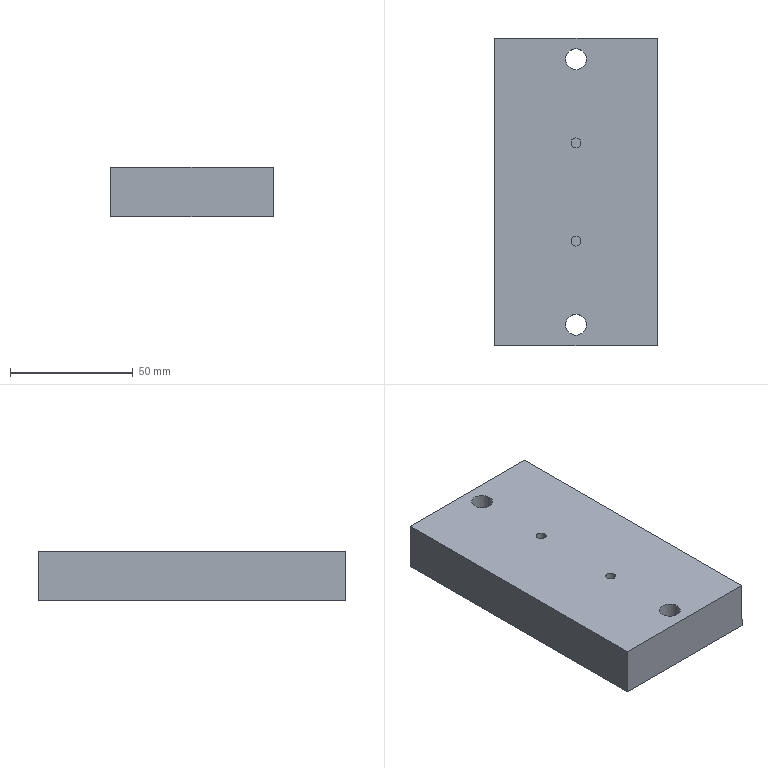Part | NX | 1 solid | 12 faces | box 65.936 x 125 x 20 mm | volume 162319 mm3 | plane 8 | cylinder 4 | commonest cylinder face diameters 4 x2 8.5 x2
STEP:
#1=CARTESIAN_POINT('',(32.535,-62.5,-63.425));
#2=VERTEX_POINT('',#1);
#3=CARTESIAN_POINT('',(32.535,62.5,-63.425));
#4=VERTEX_POINT('',#3);
#5=CARTESIAN_POINT('',(32.535,0.,-63.425));
#6=DIRECTION('',(0.,1.,0.));
#7=VECTOR('',#6,1000.);
#8=LINE('',#5,#7);
#9=EDGE_CURVE('',#2,#4,#8,.T.);
#10=ORIENTED_EDGE('',*,*,#9,.F.);
#11=CARTESIAN_POINT('',(32.535,-62.5,-83.425));
#12=VERTEX_POINT('',#11);
#13=CARTESIAN_POINT('',(32.535,-62.5,-83.425));
#14=DIRECTION('',(0.,0.,1.));
#15=VECTOR('',#14,1000.);
#16=LINE('',#13,#15);
#17=EDGE_CURVE('',#12,#2,#16,.T.);
#18=ORIENTED_EDGE('',*,*,#17,.F.);
#19=CARTESIAN_POINT('',(32.535,62.5,-83.425));
#20=VERTEX_POINT('',#19);
#21=CARTESIAN_POINT('',(32.535,-62.5,-83.425));
#22=DIRECTION('',(0.,1.,0.));
#23=VECTOR('',#22,1000.);
#24=LINE('',#21,#23);
#25=EDGE_CURVE('',#12,#20,#24,.T.);
#26=ORIENTED_EDGE('',*,*,#25,.T.);
#27=CARTESIAN_POINT('',(32.535,62.5,-83.425));
#28=DIRECTION('',(0.,0.,1.));
#29=VECTOR('',#28,1000.);
#30=LINE('',#27,#29);
#31=EDGE_CURVE('',#20,#4,#30,.T.);
#32=ORIENTED_EDGE('',*,*,#31,.T.);
#33=EDGE_LOOP('',(#10,#18,#26,#32));
#34=FACE_BOUND('',#33,.T.);
#35=CARTESIAN_POINT('',(32.535,-62.5,-83.425));
#36=DIRECTION('',(1.,0.,0.));
#37=DIRECTION('',(0.,1.,0.));
#38=AXIS2_PLACEMENT_3D('',#35,#36,#37);
#39=PLANE('',#38);
#40=ADVANCED_FACE('',(#34),#39,.T.);
#41=CARTESIAN_POINT('',(-33.401,62.5,-63.425));
#42=VERTEX_POINT('',#41);
#43=CARTESIAN_POINT('',(0.,62.5,-63.425));
#44=DIRECTION('',(-1.,0.,0.));
#45=VECTOR('',#44,1000.);
#46=LINE('',#43,#45);
#47=EDGE_CURVE('',#4,#42,#46,.T.);
#48=ORIENTED_EDGE('',*,*,#47,.F.);
#49=ORIENTED_EDGE('',*,*,#31,.F.);
#50=CARTESIAN_POINT('',(-33.401,62.5,-83.425));
#51=VERTEX_POINT('',#50);
#52=CARTESIAN_POINT('',(32.535,62.5,-83.425));
#53=DIRECTION('',(-1.,0.,0.));
#54=VECTOR('',#53,1000.);
#55=LINE('',#52,#54);
#56=EDGE_CURVE('',#20,#51,#55,.T.);
#57=ORIENTED_EDGE('',*,*,#56,.T.);
#58=CARTESIAN_POINT('',(-33.401,62.5,-83.425));
#59=DIRECTION('',(0.,0.,1.));
#60=VECTOR('',#59,1000.);
#61=LINE('',#58,#60);
#62=EDGE_CURVE('',#51,#42,#61,.T.);
#63=ORIENTED_EDGE('',*,*,#62,.T.);
#64=EDGE_LOOP('',(#48,#49,#57,#63));
#65=FACE_BOUND('',#64,.T.);
#66=CARTESIAN_POINT('',(32.535,62.5,-83.425));
#67=DIRECTION('',(0.,1.,0.));
#68=DIRECTION('',(-1.,0.,0.));
#69=AXIS2_PLACEMENT_3D('',#66,#67,#68);
#70=PLANE('',#69);
#71=ADVANCED_FACE('',(#65),#70,.T.);
#72=CARTESIAN_POINT('',(-33.401,-62.5,-63.425));
#73=VERTEX_POINT('',#72);
#74=CARTESIAN_POINT('',(-33.401,0.,-63.425));
#75=DIRECTION('',(0.,-1.,0.));
#76=VECTOR('',#75,1000.);
#77=LINE('',#74,#76);
#78=EDGE_CURVE('',#42,#73,#77,.T.);
#79=ORIENTED_EDGE('',*,*,#78,.F.);
#80=ORIENTED_EDGE('',*,*,#62,.F.);
#81=CARTESIAN_POINT('',(-33.401,-62.5,-83.425));
#82=VERTEX_POINT('',#81);
#83=CARTESIAN_POINT('',(-33.401,62.5,-83.425));
#84=DIRECTION('',(0.,-1.,0.));
#85=VECTOR('',#84,1000.);
#86=LINE('',#83,#85);
#87=EDGE_CURVE('',#51,#82,#86,.T.);
#88=ORIENTED_EDGE('',*,*,#87,.T.);
#89=CARTESIAN_POINT('',(-33.401,-62.5,-83.425));
#90=DIRECTION('',(0.,0.,1.));
#91=VECTOR('',#90,1000.);
#92=LINE('',#89,#91);
#93=EDGE_CURVE('',#82,#73,#92,.T.);
#94=ORIENTED_EDGE('',*,*,#93,.T.);
#95=EDGE_LOOP('',(#79,#80,#88,#94));
#96=FACE_BOUND('',#95,.T.);
#97=CARTESIAN_POINT('',(-33.401,62.5,-83.425));
#98=DIRECTION('',(-1.,0.,0.));
#99=DIRECTION('',(0.,-1.,0.));
#100=AXIS2_PLACEMENT_3D('',#97,#98,#99);
#101=PLANE('',#100);
#102=ADVANCED_FACE('',(#96),#101,.T.);
#103=CARTESIAN_POINT('',(0.,-62.5,-63.425));
#104=DIRECTION('',(1.,0.,0.));
#105=VECTOR('',#104,1000.);
#106=LINE('',#103,#105);
#107=EDGE_CURVE('',#73,#2,#106,.T.);
#108=ORIENTED_EDGE('',*,*,#107,.F.);
#109=ORIENTED_EDGE('',*,*,#93,.F.);
#110=CARTESIAN_POINT('',(-33.401,-62.5,-83.425));
#111=DIRECTION('',(1.,0.,0.));
#112=VECTOR('',#111,1000.);
#113=LINE('',#110,#112);
#114=EDGE_CURVE('',#82,#12,#113,.T.);
#115=ORIENTED_EDGE('',*,*,#114,.T.);
#116=ORIENTED_EDGE('',*,*,#17,.T.);
#117=EDGE_LOOP('',(#108,#109,#115,#116));
#118=FACE_BOUND('',#117,.T.);
#119=CARTESIAN_POINT('',(-33.401,-62.5,-83.425));
#120=DIRECTION('',(0.,-1.,0.));
#121=DIRECTION('',(1.,0.,0.));
#122=AXIS2_PLACEMENT_3D('',#119,#120,#121);
#123=PLANE('',#122);
#124=ADVANCED_FACE('',(#118),#123,.T.);
#125=CARTESIAN_POINT('',(3.817,54.,-83.425));
#126=VERTEX_POINT('',#125);
#127=CARTESIAN_POINT('',(-0.4329,54.,-83.425));
#128=DIRECTION('',(0.,0.,-1.));
#129=DIRECTION('',(1.,0.,0.));
#130=AXIS2_PLACEMENT_3D('',#127,#128,#129);
#131=CIRCLE('',#130,4.25);
#132=EDGE_CURVE('',#126,#126,#131,.T.);
#133=ORIENTED_EDGE('',*,*,#132,.F.);
#134=EDGE_LOOP('',(#133));
#135=FACE_BOUND('',#134,.T.);
#136=CARTESIAN_POINT('',(3.817,-54.,-83.425));
#137=VERTEX_POINT('',#136);
#138=CARTESIAN_POINT('',(-0.4329,-54.,-83.425));
#139=DIRECTION('',(0.,0.,1.));
#140=DIRECTION('',(1.,0.,0.));
#141=AXIS2_PLACEMENT_3D('',#138,#139,#140);
#142=CIRCLE('',#141,4.25);
#143=EDGE_CURVE('',#137,#137,#142,.T.);
#144=ORIENTED_EDGE('',*,*,#143,.T.);
#145=EDGE_LOOP('',(#144));
#146=FACE_BOUND('',#145,.T.);
#147=ORIENTED_EDGE('',*,*,#25,.F.);
#148=ORIENTED_EDGE('',*,*,#114,.F.);
#149=ORIENTED_EDGE('',*,*,#87,.F.);
#150=ORIENTED_EDGE('',*,*,#56,.F.);
#151=EDGE_LOOP('',(#147,#148,#149,#150));
#152=FACE_BOUND('',#151,.T.);
#153=CARTESIAN_POINT('',(0.,0.,-83.425));
#154=DIRECTION('',(0.,0.,1.));
#155=DIRECTION('',(1.,0.,0.));
#156=AXIS2_PLACEMENT_3D('',#153,#154,#155);
#157=PLANE('',#156);
#158=ADVANCED_FACE('',(#135,#146,#152),#157,.F.);
#159=CARTESIAN_POINT('',(-0.4329,-22.,-63.425));
#160=VERTEX_POINT('',#159);
#161=CARTESIAN_POINT('',(-0.4329,-20.,-63.425));
#162=DIRECTION('',(0.,0.,1.));
#163=DIRECTION('',(0.,-1.,0.));
#164=AXIS2_PLACEMENT_3D('',#161,#162,#163);
#165=CIRCLE('',#164,2.);
#166=EDGE_CURVE('',#160,#160,#165,.F.);
#167=ORIENTED_EDGE('',*,*,#166,.T.);
#168=EDGE_LOOP('',(#167));
#169=FACE_BOUND('',#168,.T.);
#170=CARTESIAN_POINT('',(-0.4329,18.,-63.425));
#171=VERTEX_POINT('',#170);
#172=CARTESIAN_POINT('',(-0.4329,20.,-63.425));
#173=DIRECTION('',(0.,0.,1.));
#174=DIRECTION('',(0.,-1.,0.));
#175=AXIS2_PLACEMENT_3D('',#172,#173,#174);
#176=CIRCLE('',#175,2.);
#177=EDGE_CURVE('',#171,#171,#176,.F.);
#178=ORIENTED_EDGE('',*,*,#177,.T.);
#179=EDGE_LOOP('',(#178));
#180=FACE_BOUND('',#179,.T.);
#181=CARTESIAN_POINT('',(3.817,-54.,-63.425));
#182=VERTEX_POINT('',#181);
#183=CARTESIAN_POINT('',(-0.4329,-54.,-63.425));
#184=DIRECTION('',(0.,0.,1.));
#185=DIRECTION('',(1.,0.,0.));
#186=AXIS2_PLACEMENT_3D('',#183,#184,#185);
#187=CIRCLE('',#186,4.25);
#188=EDGE_CURVE('',#182,#182,#187,.F.);
#189=ORIENTED_EDGE('',*,*,#188,.T.);
#190=EDGE_LOOP('',(#189));
#191=FACE_BOUND('',#190,.T.);
#192=CARTESIAN_POINT('',(3.817,54.,-63.425));
#193=VERTEX_POINT('',#192);
#194=CARTESIAN_POINT('',(-0.4329,54.,-63.425));
#195=DIRECTION('',(0.,0.,1.));
#196=DIRECTION('',(1.,0.,0.));
#197=AXIS2_PLACEMENT_3D('',#194,#195,#196);
#198=CIRCLE('',#197,4.25);
#199=EDGE_CURVE('',#193,#193,#198,.F.);
#200=ORIENTED_EDGE('',*,*,#199,.T.);
#201=EDGE_LOOP('',(#200));
#202=FACE_BOUND('',#201,.T.);
#203=ORIENTED_EDGE('',*,*,#47,.T.);
#204=ORIENTED_EDGE('',*,*,#78,.T.);
#205=ORIENTED_EDGE('',*,*,#107,.T.);
#206=ORIENTED_EDGE('',*,*,#9,.T.);
#207=EDGE_LOOP('',(#203,#204,#205,#206));
#208=FACE_BOUND('',#207,.T.);
#209=CARTESIAN_POINT('',(0.,0.,-63.425));
#210=DIRECTION('',(0.,0.,1.));
#211=DIRECTION('',(1.,0.,0.));
#212=AXIS2_PLACEMENT_3D('',#209,#210,#211);
#213=PLANE('',#212);
#214=ADVANCED_FACE('',(#169,#180,#191,#202,#208),#213,.T.);
#215=ORIENTED_EDGE('',*,*,#166,.F.);
#216=EDGE_LOOP('',(#215));
#217=FACE_BOUND('',#216,.T.);
#218=CARTESIAN_POINT('',(-0.4329,-22.,-73.425));
#219=VERTEX_POINT('',#218);
#220=CARTESIAN_POINT('',(-0.4329,-20.,-73.425));
#221=DIRECTION('',(0.,0.,-1.));
#222=DIRECTION('',(0.,-1.,0.));
#223=AXIS2_PLACEMENT_3D('',#220,#221,#222);
#224=CIRCLE('',#223,2.);
#225=EDGE_CURVE('',#219,#219,#224,.F.);
#226=ORIENTED_EDGE('',*,*,#225,.F.);
#227=EDGE_LOOP('',(#226));
#228=FACE_BOUND('',#227,.T.);
#229=CARTESIAN_POINT('',(-0.4329,-20.,-73.425));
#230=DIRECTION('',(0.,0.,1.));
#231=DIRECTION('',(1.,0.,0.));
#232=AXIS2_PLACEMENT_3D('',#229,#230,#231);
#233=CYLINDRICAL_SURFACE('',#232,2.);
#234=ADVANCED_FACE('',(#217,#228),#233,.F.);
#235=ORIENTED_EDGE('',*,*,#225,.T.);
#236=EDGE_LOOP('',(#235));
#237=FACE_BOUND('',#236,.T.);
#238=CARTESIAN_POINT('',(-0.4329,-20.,-73.425));
#239=DIRECTION('',(0.,0.,-1.));
#240=DIRECTION('',(-1.,0.,0.));
#241=AXIS2_PLACEMENT_3D('',#238,#239,#240);
#242=PLANE('',#241);
#243=ADVANCED_FACE('',(#237),#242,.F.);
#244=ORIENTED_EDGE('',*,*,#177,.F.);
#245=EDGE_LOOP('',(#244));
#246=FACE_BOUND('',#245,.T.);
#247=CARTESIAN_POINT('',(-0.4329,18.,-73.425));
#248=VERTEX_POINT('',#247);
#249=CARTESIAN_POINT('',(-0.4329,20.,-73.425));
#250=DIRECTION('',(0.,0.,-1.));
#251=DIRECTION('',(0.,-1.,0.));
#252=AXIS2_PLACEMENT_3D('',#249,#250,#251);
#253=CIRCLE('',#252,2.);
#254=EDGE_CURVE('',#248,#248,#253,.F.);
#255=ORIENTED_EDGE('',*,*,#254,.F.);
#256=EDGE_LOOP('',(#255));
#257=FACE_BOUND('',#256,.T.);
#258=CARTESIAN_POINT('',(-0.4329,20.,-73.425));
#259=DIRECTION('',(0.,0.,1.));
#260=DIRECTION('',(1.,0.,0.));
#261=AXIS2_PLACEMENT_3D('',#258,#259,#260);
#262=CYLINDRICAL_SURFACE('',#261,2.);
#263=ADVANCED_FACE('',(#246,#257),#262,.F.);
#264=ORIENTED_EDGE('',*,*,#254,.T.);
#265=EDGE_LOOP('',(#264));
#266=FACE_BOUND('',#265,.T.);
#267=CARTESIAN_POINT('',(-0.4329,20.,-73.425));
#268=DIRECTION('',(0.,0.,-1.));
#269=DIRECTION('',(-1.,0.,0.));
#270=AXIS2_PLACEMENT_3D('',#267,#268,#269);
#271=PLANE('',#270);
#272=ADVANCED_FACE('',(#266),#271,.F.);
#273=ORIENTED_EDGE('',*,*,#143,.F.);
#274=EDGE_LOOP('',(#273));
#275=FACE_BOUND('',#274,.T.);
#276=ORIENTED_EDGE('',*,*,#188,.F.);
#277=EDGE_LOOP('',(#276));
#278=FACE_BOUND('',#277,.T.);
#279=CARTESIAN_POINT('',(-0.4329,-54.,-83.425));
#280=DIRECTION('',(0.,0.,1.));
#281=DIRECTION('',(1.,0.,0.));
#282=AXIS2_PLACEMENT_3D('',#279,#280,#281);
#283=CYLINDRICAL_SURFACE('',#282,4.25);
#284=ADVANCED_FACE('',(#275,#278),#283,.F.);
#285=ORIENTED_EDGE('',*,*,#199,.F.);
#286=EDGE_LOOP('',(#285));
#287=FACE_BOUND('',#286,.T.);
#288=ORIENTED_EDGE('',*,*,#132,.T.);
#289=EDGE_LOOP('',(#288));
#290=FACE_BOUND('',#289,.T.);
#291=CARTESIAN_POINT('',(-0.4329,54.,-83.425));
#292=DIRECTION('',(0.,0.,1.));
#293=DIRECTION('',(1.,0.,0.));
#294=AXIS2_PLACEMENT_3D('',#291,#292,#293);
#295=CYLINDRICAL_SURFACE('',#294,4.25);
#296=ADVANCED_FACE('',(#287,#290),#295,.F.);
#297=CLOSED_SHELL('',(#40,#71,#102,#124,#158,#214,#234,#243,#263,#272,#284,#296));
#298=MANIFOLD_SOLID_BREP('',#297);
#299=(LENGTH_UNIT()NAMED_UNIT(*)SI_UNIT(.MILLI.,.METRE.));
#300=UNCERTAINTY_MEASURE_WITH_UNIT(LENGTH_MEASURE(0.00001),#299,'','');
#301=(NAMED_UNIT(*)PLANE_ANGLE_UNIT()SI_UNIT($,.RADIAN.));
#302=(NAMED_UNIT(*)SI_UNIT($,.STERADIAN.)SOLID_ANGLE_UNIT());
#303=(GEOMETRIC_REPRESENTATION_CONTEXT(3)GLOBAL_UNCERTAINTY_ASSIGNED_CONTEXT((#300))GLOBAL_UNIT_ASSIGNED_CONTEXT((#299,#301,#302))REPRESENTATION_CONTEXT('',''));
#304=ADVANCED_BREP_SHAPE_REPRESENTATION('',(#298),#303);